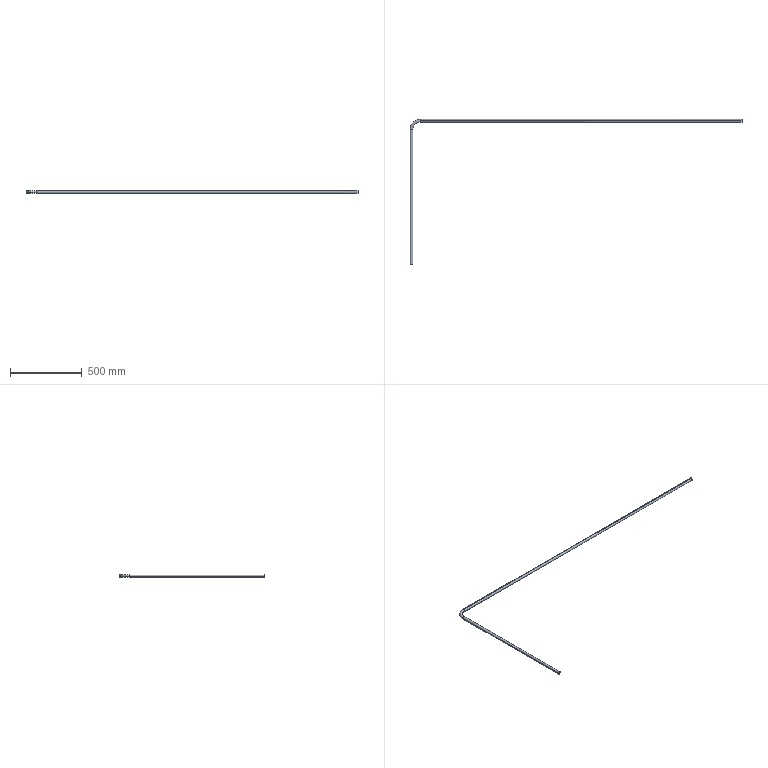Part | SolidWorks | features Sweep 1 | 1 solid | 14 faces | box 2310 x 1010 x 20 mm | volume 370309 mm3 | cylinder 8 | torus 4 | plane 2 | commonest cylinder face diameters 16 x4 20 x4
STEP:
#1=CARTESIAN_POINT('',(60.,0.,-8.));
#2=VERTEX_POINT('',#1);
#3=CARTESIAN_POINT('',(60.,8.,0.));
#4=VERTEX_POINT('',#3);
#5=CARTESIAN_POINT('',(60.,0.,0.));
#6=DIRECTION('',(1.,0.,0.));
#7=DIRECTION('',(0.,0.,1.));
#8=AXIS2_PLACEMENT_3D('',#5,#6,#7);
#9=CIRCLE('',#8,8.);
#10=EDGE_CURVE('',#2,#4,#9,.T.);
#11=ORIENTED_EDGE('',*,*,#10,.T.);
#12=CARTESIAN_POINT('',(-8.,-60.,0.));
#13=VERTEX_POINT('',#12);
#14=CARTESIAN_POINT('',(60.,-60.,0.));
#15=DIRECTION('',(0.,0.,1.));
#16=DIRECTION('',(1.,0.,0.));
#17=AXIS2_PLACEMENT_3D('',#14,#15,#16);
#18=CIRCLE('',#17,68.);
#19=EDGE_CURVE('',#4,#13,#18,.T.);
#20=ORIENTED_EDGE('',*,*,#19,.T.);
#21=CARTESIAN_POINT('',(8.,-60.,0.));
#22=VERTEX_POINT('',#21);
#23=CARTESIAN_POINT('',(0.,-60.,0.));
#24=DIRECTION('',(0.,1.,0.));
#25=DIRECTION('',(-1.,0.,0.));
#26=AXIS2_PLACEMENT_3D('',#23,#24,#25);
#27=CIRCLE('',#26,8.);
#28=EDGE_CURVE('',#22,#13,#27,.T.);
#29=ORIENTED_EDGE('',*,*,#28,.F.);
#30=CARTESIAN_POINT('',(60.,-8.,0.));
#31=VERTEX_POINT('',#30);
#32=CARTESIAN_POINT('',(60.,-60.,0.));
#33=DIRECTION('',(0.,0.,1.));
#34=DIRECTION('',(1.,0.,0.));
#35=AXIS2_PLACEMENT_3D('',#32,#33,#34);
#36=CIRCLE('',#35,52.);
#37=EDGE_CURVE('',#31,#22,#36,.T.);
#38=ORIENTED_EDGE('',*,*,#37,.F.);
#39=CARTESIAN_POINT('',(60.,0.,0.));
#40=DIRECTION('',(1.,0.,0.));
#41=DIRECTION('',(0.,0.,1.));
#42=AXIS2_PLACEMENT_3D('',#39,#40,#41);
#43=CIRCLE('',#42,8.);
#44=EDGE_CURVE('',#31,#2,#43,.T.);
#45=ORIENTED_EDGE('',*,*,#44,.T.);
#46=EDGE_LOOP('',(#11,#20,#29,#38,#45));
#47=FACE_OUTER_BOUND('',#46,.T.);
#48=CARTESIAN_POINT('',(60.,-60.,0.));
#49=DIRECTION('',(0.,0.,1.));
#50=DIRECTION('',(1.,0.,0.));
#51=AXIS2_PLACEMENT_3D('',#48,#49,#50);
#52=TOROIDAL_SURFACE('',#51,60.,8.);
#53=ADVANCED_FACE('',(#47),#52,.F.);
#54=CARTESIAN_POINT('',(60.,10.,0.));
#55=VERTEX_POINT('',#54);
#56=CARTESIAN_POINT('',(60.,0.,10.));
#57=VERTEX_POINT('',#56);
#58=CARTESIAN_POINT('',(60.,0.,0.));
#59=DIRECTION('',(1.,0.,0.));
#60=DIRECTION('',(0.,1.,0.));
#61=AXIS2_PLACEMENT_3D('',#58,#59,#60);
#62=CIRCLE('',#61,10.);
#63=EDGE_CURVE('',#55,#57,#62,.T.);
#64=ORIENTED_EDGE('',*,*,#63,.F.);
#65=CARTESIAN_POINT('',(-10.,-60.,0.));
#66=VERTEX_POINT('',#65);
#67=CARTESIAN_POINT('',(60.,-60.,0.));
#68=DIRECTION('',(0.,0.,1.));
#69=DIRECTION('',(1.,0.,0.));
#70=AXIS2_PLACEMENT_3D('',#67,#68,#69);
#71=CIRCLE('',#70,70.);
#72=EDGE_CURVE('',#55,#66,#71,.T.);
#73=ORIENTED_EDGE('',*,*,#72,.T.);
#74=CARTESIAN_POINT('',(10.,-60.,0.));
#75=VERTEX_POINT('',#74);
#76=CARTESIAN_POINT('',(0.,-60.,0.));
#77=DIRECTION('',(0.,1.,0.));
#78=DIRECTION('',(-1.,0.,0.));
#79=AXIS2_PLACEMENT_3D('',#76,#77,#78);
#80=CIRCLE('',#79,10.);
#81=EDGE_CURVE('',#66,#75,#80,.T.);
#82=ORIENTED_EDGE('',*,*,#81,.T.);
#83=CARTESIAN_POINT('',(60.,-10.,0.));
#84=VERTEX_POINT('',#83);
#85=CARTESIAN_POINT('',(60.,-60.,0.));
#86=DIRECTION('',(0.,0.,1.));
#87=DIRECTION('',(1.,0.,0.));
#88=AXIS2_PLACEMENT_3D('',#85,#86,#87);
#89=CIRCLE('',#88,50.);
#90=EDGE_CURVE('',#84,#75,#89,.T.);
#91=ORIENTED_EDGE('',*,*,#90,.F.);
#92=CARTESIAN_POINT('',(60.,0.,0.));
#93=DIRECTION('',(1.,0.,0.));
#94=DIRECTION('',(0.,1.,0.));
#95=AXIS2_PLACEMENT_3D('',#92,#93,#94);
#96=CIRCLE('',#95,10.);
#97=EDGE_CURVE('',#57,#84,#96,.T.);
#98=ORIENTED_EDGE('',*,*,#97,.F.);
#99=EDGE_LOOP('',(#64,#73,#82,#91,#98));
#100=FACE_OUTER_BOUND('',#99,.T.);
#101=CARTESIAN_POINT('',(60.,-60.,0.));
#102=DIRECTION('',(0.,0.,1.));
#103=DIRECTION('',(1.,0.,0.));
#104=AXIS2_PLACEMENT_3D('',#101,#102,#103);
#105=TOROIDAL_SURFACE('',#104,60.,10.);
#106=ADVANCED_FACE('',(#100),#105,.T.);
#107=ORIENTED_EDGE('',*,*,#28,.T.);
#108=CARTESIAN_POINT('',(-8.,-1000.,0.));
#109=VERTEX_POINT('',#108);
#110=CARTESIAN_POINT('',(-8.,-60.,0.));
#111=DIRECTION('',(0.,-1.,0.));
#112=VECTOR('',#111,1000.);
#113=LINE('',#110,#112);
#114=EDGE_CURVE('',#13,#109,#113,.T.);
#115=ORIENTED_EDGE('',*,*,#114,.T.);
#116=CARTESIAN_POINT('',(8.,-1000.,0.));
#117=VERTEX_POINT('',#116);
#118=CARTESIAN_POINT('',(0.,-1000.,0.));
#119=DIRECTION('',(0.,1.,0.));
#120=DIRECTION('',(-1.,0.,0.));
#121=AXIS2_PLACEMENT_3D('',#118,#119,#120);
#122=CIRCLE('',#121,8.);
#123=EDGE_CURVE('',#117,#109,#122,.T.);
#124=ORIENTED_EDGE('',*,*,#123,.F.);
#125=CARTESIAN_POINT('',(8.,-60.,0.));
#126=DIRECTION('',(0.,-1.,0.));
#127=VECTOR('',#126,1000.);
#128=LINE('',#125,#127);
#129=EDGE_CURVE('',#22,#117,#128,.T.);
#130=ORIENTED_EDGE('',*,*,#129,.F.);
#131=EDGE_LOOP('',(#107,#115,#124,#130));
#132=FACE_OUTER_BOUND('',#131,.T.);
#133=CARTESIAN_POINT('',(0.,-60.,0.));
#134=DIRECTION('',(0.,-1.,0.));
#135=DIRECTION('',(1.,0.,0.));
#136=AXIS2_PLACEMENT_3D('',#133,#134,#135);
#137=CYLINDRICAL_SURFACE('',#136,8.);
#138=ADVANCED_FACE('',(#132),#137,.F.);
#139=CARTESIAN_POINT('',(2300.,0.,8.));
#140=VERTEX_POINT('',#139);
#141=CARTESIAN_POINT('',(2300.,0.,-8.));
#142=VERTEX_POINT('',#141);
#143=CARTESIAN_POINT('',(2300.,0.,0.));
#144=DIRECTION('',(1.,0.,0.));
#145=DIRECTION('',(0.,1.,0.));
#146=AXIS2_PLACEMENT_3D('',#143,#144,#145);
#147=CIRCLE('',#146,8.);
#148=EDGE_CURVE('',#140,#142,#147,.T.);
#149=ORIENTED_EDGE('',*,*,#148,.T.);
#150=CARTESIAN_POINT('',(2300.,0.,-8.));
#151=DIRECTION('',(-1.,0.,0.));
#152=VECTOR('',#151,1000.);
#153=LINE('',#150,#152);
#154=EDGE_CURVE('',#142,#2,#153,.T.);
#155=ORIENTED_EDGE('',*,*,#154,.T.);
#156=ORIENTED_EDGE('',*,*,#44,.F.);
#157=CARTESIAN_POINT('',(60.,0.,8.));
#158=VERTEX_POINT('',#157);
#159=CARTESIAN_POINT('',(60.,0.,0.));
#160=DIRECTION('',(1.,0.,0.));
#161=DIRECTION('',(0.,0.,1.));
#162=AXIS2_PLACEMENT_3D('',#159,#160,#161);
#163=CIRCLE('',#162,8.);
#164=EDGE_CURVE('',#158,#31,#163,.T.);
#165=ORIENTED_EDGE('',*,*,#164,.F.);
#166=CARTESIAN_POINT('',(2300.,0.,8.));
#167=DIRECTION('',(-1.,0.,0.));
#168=VECTOR('',#167,1000.);
#169=LINE('',#166,#168);
#170=EDGE_CURVE('',#140,#158,#169,.T.);
#171=ORIENTED_EDGE('',*,*,#170,.F.);
#172=EDGE_LOOP('',(#149,#155,#156,#165,#171));
#173=FACE_OUTER_BOUND('',#172,.T.);
#174=CARTESIAN_POINT('',(2300.,0.,0.));
#175=DIRECTION('',(-1.,0.,0.));
#176=DIRECTION('',(0.,0.,1.));
#177=AXIS2_PLACEMENT_3D('',#174,#175,#176);
#178=CYLINDRICAL_SURFACE('',#177,8.);
#179=ADVANCED_FACE('',(#173),#178,.F.);
#180=ORIENTED_EDGE('',*,*,#81,.F.);
#181=CARTESIAN_POINT('',(-10.,-1000.,0.));
#182=VERTEX_POINT('',#181);
#183=CARTESIAN_POINT('',(-10.,-60.,0.));
#184=DIRECTION('',(0.,-1.,0.));
#185=VECTOR('',#184,1000.);
#186=LINE('',#183,#185);
#187=EDGE_CURVE('',#66,#182,#186,.T.);
#188=ORIENTED_EDGE('',*,*,#187,.T.);
#189=CARTESIAN_POINT('',(10.,-1000.,0.));
#190=VERTEX_POINT('',#189);
#191=CARTESIAN_POINT('',(0.,-1000.,0.));
#192=DIRECTION('',(0.,1.,0.));
#193=DIRECTION('',(-1.,0.,0.));
#194=AXIS2_PLACEMENT_3D('',#191,#192,#193);
#195=CIRCLE('',#194,10.);
#196=EDGE_CURVE('',#182,#190,#195,.T.);
#197=ORIENTED_EDGE('',*,*,#196,.T.);
#198=CARTESIAN_POINT('',(10.,-60.,0.));
#199=DIRECTION('',(0.,-1.,0.));
#200=VECTOR('',#199,1000.);
#201=LINE('',#198,#200);
#202=EDGE_CURVE('',#75,#190,#201,.T.);
#203=ORIENTED_EDGE('',*,*,#202,.F.);
#204=EDGE_LOOP('',(#180,#188,#197,#203));
#205=FACE_OUTER_BOUND('',#204,.T.);
#206=CARTESIAN_POINT('',(0.,-60.,0.));
#207=DIRECTION('',(0.,-1.,0.));
#208=DIRECTION('',(1.,0.,0.));
#209=AXIS2_PLACEMENT_3D('',#206,#207,#208);
#210=CYLINDRICAL_SURFACE('',#209,10.);
#211=ADVANCED_FACE('',(#205),#210,.T.);
#212=CARTESIAN_POINT('',(2300.,0.,-10.));
#213=VERTEX_POINT('',#212);
#214=CARTESIAN_POINT('',(2300.,0.,10.));
#215=VERTEX_POINT('',#214);
#216=CARTESIAN_POINT('',(2300.,0.,0.));
#217=DIRECTION('',(1.,0.,0.));
#218=DIRECTION('',(0.,1.,0.));
#219=AXIS2_PLACEMENT_3D('',#216,#217,#218);
#220=CIRCLE('',#219,10.);
#221=EDGE_CURVE('',#213,#215,#220,.T.);
#222=ORIENTED_EDGE('',*,*,#221,.F.);
#223=CARTESIAN_POINT('',(60.,0.,-10.));
#224=VERTEX_POINT('',#223);
#225=CARTESIAN_POINT('',(2300.,0.,-10.));
#226=DIRECTION('',(-1.,0.,0.));
#227=VECTOR('',#226,1000.);
#228=LINE('',#225,#227);
#229=EDGE_CURVE('',#213,#224,#228,.T.);
#230=ORIENTED_EDGE('',*,*,#229,.T.);
#231=CARTESIAN_POINT('',(60.,0.,0.));
#232=DIRECTION('',(1.,0.,0.));
#233=DIRECTION('',(0.,1.,0.));
#234=AXIS2_PLACEMENT_3D('',#231,#232,#233);
#235=CIRCLE('',#234,10.);
#236=EDGE_CURVE('',#224,#55,#235,.T.);
#237=ORIENTED_EDGE('',*,*,#236,.T.);
#238=ORIENTED_EDGE('',*,*,#63,.T.);
#239=CARTESIAN_POINT('',(2300.,0.,10.));
#240=DIRECTION('',(-1.,0.,0.));
#241=VECTOR('',#240,1000.);
#242=LINE('',#239,#241);
#243=EDGE_CURVE('',#215,#57,#242,.T.);
#244=ORIENTED_EDGE('',*,*,#243,.F.);
#245=EDGE_LOOP('',(#222,#230,#237,#238,#244));
#246=FACE_OUTER_BOUND('',#245,.T.);
#247=CARTESIAN_POINT('',(2300.,0.,0.));
#248=DIRECTION('',(-1.,0.,0.));
#249=DIRECTION('',(0.,0.,1.));
#250=AXIS2_PLACEMENT_3D('',#247,#248,#249);
#251=CYLINDRICAL_SURFACE('',#250,10.);
#252=ADVANCED_FACE('',(#246),#251,.T.);
#253=ORIENTED_EDGE('',*,*,#187,.F.);
#254=CARTESIAN_POINT('',(0.,-60.,0.));
#255=DIRECTION('',(0.,1.,0.));
#256=DIRECTION('',(-1.,0.,0.));
#257=AXIS2_PLACEMENT_3D('',#254,#255,#256);
#258=CIRCLE('',#257,10.);
#259=EDGE_CURVE('',#75,#66,#258,.T.);
#260=ORIENTED_EDGE('',*,*,#259,.F.);
#261=ORIENTED_EDGE('',*,*,#202,.T.);
#262=CARTESIAN_POINT('',(0.,-1000.,0.));
#263=DIRECTION('',(0.,1.,0.));
#264=DIRECTION('',(-1.,0.,0.));
#265=AXIS2_PLACEMENT_3D('',#262,#263,#264);
#266=CIRCLE('',#265,10.);
#267=EDGE_CURVE('',#190,#182,#266,.T.);
#268=ORIENTED_EDGE('',*,*,#267,.T.);
#269=EDGE_LOOP('',(#253,#260,#261,#268));
#270=FACE_OUTER_BOUND('',#269,.T.);
#271=CARTESIAN_POINT('',(0.,-60.,0.));
#272=DIRECTION('',(0.,-1.,0.));
#273=DIRECTION('',(1.,0.,0.));
#274=AXIS2_PLACEMENT_3D('',#271,#272,#273);
#275=CYLINDRICAL_SURFACE('',#274,10.);
#276=ADVANCED_FACE('',(#270),#275,.T.);
#277=ORIENTED_EDGE('',*,*,#72,.F.);
#278=ORIENTED_EDGE('',*,*,#236,.F.);
#279=CARTESIAN_POINT('',(60.,0.,0.));
#280=DIRECTION('',(1.,0.,0.));
#281=DIRECTION('',(0.,1.,0.));
#282=AXIS2_PLACEMENT_3D('',#279,#280,#281);
#283=CIRCLE('',#282,10.);
#284=EDGE_CURVE('',#84,#224,#283,.T.);
#285=ORIENTED_EDGE('',*,*,#284,.F.);
#286=ORIENTED_EDGE('',*,*,#90,.T.);
#287=ORIENTED_EDGE('',*,*,#259,.T.);
#288=EDGE_LOOP('',(#277,#278,#285,#286,#287));
#289=FACE_OUTER_BOUND('',#288,.T.);
#290=CARTESIAN_POINT('',(60.,-60.,0.));
#291=DIRECTION('',(0.,0.,1.));
#292=DIRECTION('',(1.,0.,0.));
#293=AXIS2_PLACEMENT_3D('',#290,#291,#292);
#294=TOROIDAL_SURFACE('',#293,60.,10.);
#295=ADVANCED_FACE('',(#289),#294,.T.);
#296=ORIENTED_EDGE('',*,*,#229,.F.);
#297=CARTESIAN_POINT('',(2300.,0.,0.));
#298=DIRECTION('',(1.,0.,0.));
#299=DIRECTION('',(0.,1.,0.));
#300=AXIS2_PLACEMENT_3D('',#297,#298,#299);
#301=CIRCLE('',#300,10.);
#302=EDGE_CURVE('',#215,#213,#301,.T.);
#303=ORIENTED_EDGE('',*,*,#302,.F.);
#304=ORIENTED_EDGE('',*,*,#243,.T.);
#305=ORIENTED_EDGE('',*,*,#97,.T.);
#306=ORIENTED_EDGE('',*,*,#284,.T.);
#307=EDGE_LOOP('',(#296,#303,#304,#305,#306));
#308=FACE_OUTER_BOUND('',#307,.T.);
#309=CARTESIAN_POINT('',(2300.,0.,0.));
#310=DIRECTION('',(-1.,0.,0.));
#311=DIRECTION('',(0.,0.,1.));
#312=AXIS2_PLACEMENT_3D('',#309,#310,#311);
#313=CYLINDRICAL_SURFACE('',#312,10.);
#314=ADVANCED_FACE('',(#308),#313,.T.);
#315=ORIENTED_EDGE('',*,*,#123,.T.);
#316=CARTESIAN_POINT('',(0.,-1000.,0.));
#317=DIRECTION('',(0.,1.,0.));
#318=DIRECTION('',(-1.,0.,0.));
#319=AXIS2_PLACEMENT_3D('',#316,#317,#318);
#320=CIRCLE('',#319,8.);
#321=EDGE_CURVE('',#109,#117,#320,.T.);
#322=ORIENTED_EDGE('',*,*,#321,.T.);
#323=EDGE_LOOP('',(#315,#322));
#324=FACE_BOUND('',#323,.T.);
#325=ORIENTED_EDGE('',*,*,#267,.F.);
#326=ORIENTED_EDGE('',*,*,#196,.F.);
#327=EDGE_LOOP('',(#325,#326));
#328=FACE_OUTER_BOUND('',#327,.T.);
#329=CARTESIAN_POINT('',(0.,-1000.,0.));
#330=DIRECTION('',(0.,1.,0.));
#331=DIRECTION('',(-1.,0.,0.));
#332=AXIS2_PLACEMENT_3D('',#329,#330,#331);
#333=PLANE('',#332);
#334=ADVANCED_FACE('',(#324,#328),#333,.F.);
#335=ORIENTED_EDGE('',*,*,#148,.F.);
#336=CARTESIAN_POINT('',(2300.,0.,0.));
#337=DIRECTION('',(1.,0.,0.));
#338=DIRECTION('',(0.,1.,0.));
#339=AXIS2_PLACEMENT_3D('',#336,#337,#338);
#340=CIRCLE('',#339,8.);
#341=EDGE_CURVE('',#142,#140,#340,.T.);
#342=ORIENTED_EDGE('',*,*,#341,.F.);
#343=EDGE_LOOP('',(#335,#342));
#344=FACE_BOUND('',#343,.T.);
#345=ORIENTED_EDGE('',*,*,#302,.T.);
#346=ORIENTED_EDGE('',*,*,#221,.T.);
#347=EDGE_LOOP('',(#345,#346));
#348=FACE_OUTER_BOUND('',#347,.T.);
#349=CARTESIAN_POINT('',(2300.,0.,0.));
#350=DIRECTION('',(1.,0.,0.));
#351=DIRECTION('',(0.,1.,0.));
#352=AXIS2_PLACEMENT_3D('',#349,#350,#351);
#353=PLANE('',#352);
#354=ADVANCED_FACE('',(#344,#348),#353,.T.);
#355=ORIENTED_EDGE('',*,*,#114,.F.);
#356=CARTESIAN_POINT('',(0.,-60.,0.));
#357=DIRECTION('',(0.,1.,0.));
#358=DIRECTION('',(-1.,0.,0.));
#359=AXIS2_PLACEMENT_3D('',#356,#357,#358);
#360=CIRCLE('',#359,8.);
#361=EDGE_CURVE('',#13,#22,#360,.T.);
#362=ORIENTED_EDGE('',*,*,#361,.T.);
#363=ORIENTED_EDGE('',*,*,#129,.T.);
#364=ORIENTED_EDGE('',*,*,#321,.F.);
#365=EDGE_LOOP('',(#355,#362,#363,#364));
#366=FACE_OUTER_BOUND('',#365,.T.);
#367=CARTESIAN_POINT('',(0.,-60.,0.));
#368=DIRECTION('',(0.,-1.,0.));
#369=DIRECTION('',(1.,0.,0.));
#370=AXIS2_PLACEMENT_3D('',#367,#368,#369);
#371=CYLINDRICAL_SURFACE('',#370,8.);
#372=ADVANCED_FACE('',(#366),#371,.F.);
#373=ORIENTED_EDGE('',*,*,#19,.F.);
#374=CARTESIAN_POINT('',(60.,0.,0.));
#375=DIRECTION('',(1.,0.,0.));
#376=DIRECTION('',(0.,0.,1.));
#377=AXIS2_PLACEMENT_3D('',#374,#375,#376);
#378=CIRCLE('',#377,8.);
#379=EDGE_CURVE('',#4,#158,#378,.T.);
#380=ORIENTED_EDGE('',*,*,#379,.T.);
#381=ORIENTED_EDGE('',*,*,#164,.T.);
#382=ORIENTED_EDGE('',*,*,#37,.T.);
#383=ORIENTED_EDGE('',*,*,#361,.F.);
#384=EDGE_LOOP('',(#373,#380,#381,#382,#383));
#385=FACE_OUTER_BOUND('',#384,.T.);
#386=CARTESIAN_POINT('',(60.,-60.,0.));
#387=DIRECTION('',(0.,0.,1.));
#388=DIRECTION('',(1.,0.,0.));
#389=AXIS2_PLACEMENT_3D('',#386,#387,#388);
#390=TOROIDAL_SURFACE('',#389,60.,8.);
#391=ADVANCED_FACE('',(#385),#390,.F.);
#392=ORIENTED_EDGE('',*,*,#154,.F.);
#393=ORIENTED_EDGE('',*,*,#341,.T.);
#394=ORIENTED_EDGE('',*,*,#170,.T.);
#395=ORIENTED_EDGE('',*,*,#379,.F.);
#396=ORIENTED_EDGE('',*,*,#10,.F.);
#397=EDGE_LOOP('',(#392,#393,#394,#395,#396));
#398=FACE_OUTER_BOUND('',#397,.T.);
#399=CARTESIAN_POINT('',(2300.,0.,0.));
#400=DIRECTION('',(-1.,0.,0.));
#401=DIRECTION('',(0.,0.,1.));
#402=AXIS2_PLACEMENT_3D('',#399,#400,#401);
#403=CYLINDRICAL_SURFACE('',#402,8.);
#404=ADVANCED_FACE('',(#398),#403,.F.);
#405=CLOSED_SHELL('',(#53,#106,#138,#179,#211,#252,#276,#295,#314,#334,#354,#372,#391,#404));
#406=MANIFOLD_SOLID_BREP('',#405);
#407=CARTESIAN_POINT('',(0.,0.,0.));
#408=DIRECTION('',(0.,0.,1.));
#409=DIRECTION('',(1.,0.,0.));
#410=AXIS2_PLACEMENT_3D('',#407,#408,#409);
#411=(LENGTH_UNIT()NAMED_UNIT(*)SI_UNIT(.MILLI.,.METRE.));
#412=UNCERTAINTY_MEASURE_WITH_UNIT(LENGTH_MEASURE(0.00001),#411,'','');
#413=(NAMED_UNIT(*)PLANE_ANGLE_UNIT()SI_UNIT($,.RADIAN.));
#414=(NAMED_UNIT(*)SI_UNIT($,.STERADIAN.)SOLID_ANGLE_UNIT());
#415=(GEOMETRIC_REPRESENTATION_CONTEXT(3)GLOBAL_UNCERTAINTY_ASSIGNED_CONTEXT((#412))GLOBAL_UNIT_ASSIGNED_CONTEXT((#411,#413,#414))REPRESENTATION_CONTEXT('',''));
#416=ADVANCED_BREP_SHAPE_REPRESENTATION('',(#406,#410),#415);